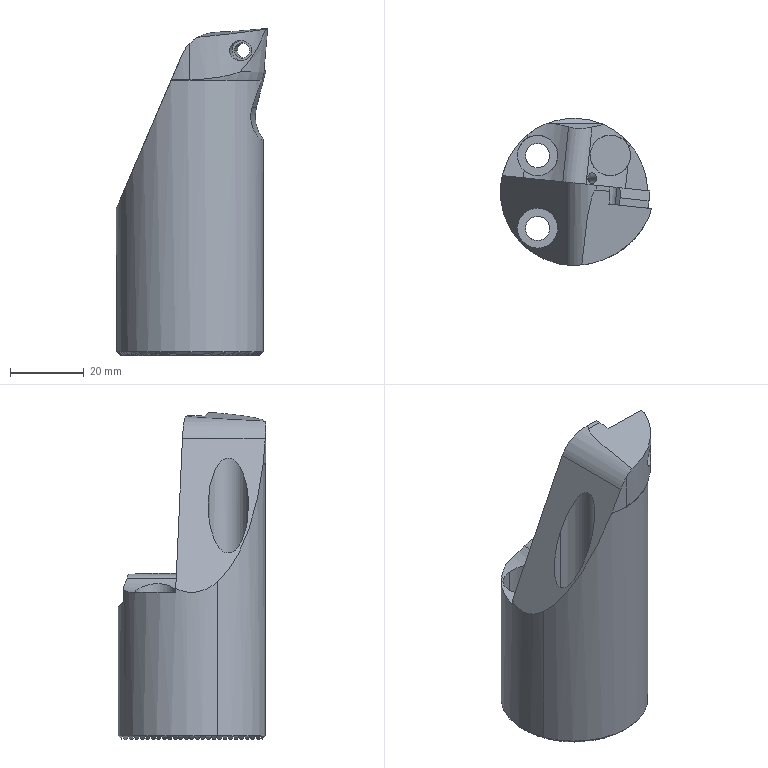NC program | Mastercam | posted with a generic post
Whole program:
%
:0001()
(MATERIAL - ALUMINUM MM - 2024)
(T8|26 60DTH |H8|D8|WEAR COMP|TOOL DIA. - 26.|XY STOCK TO LEAVE - .1|Z STOCK TO LEAVE - -.75)
(T9|12 FEMF |H9|D9|WEAR COMP|TOOL DIA. - 12.|XY STOCK TO LEAVE - .1|Z STOCK TO LEAVE - .05)
(T3|10 CHM |H3)
(T4|12 FEMR |H4|XY STOCK TO LEAVE - .15|Z STOCK TO LEAVE - .1)
N100 G21
N102 G0 G17 G40 G80 G90 G94 G98
N104 G0 G28 G91 Z0.
N106 G0 G28 X0. Y0.
(26 60DTH |TOOL - 8|DIA. OFF. - 8|LEN. - 8|TOOL DIA. - 26.)
N108 T8 M6
N110 G0 G55 G90 X17.402 Y10.083 C0. B-90. S4000 M3
N112 G43 H8 Z70.25
N114 Z21.25
N116 G1 Z14.5 F2000.
N118 G41 D8 X12.473 F1000.
N120 G3 X12.35 Y9.96 J-.123
N122 G1 Y6.96
N124 Y-6.96
N126 Y-9.96
N128 G3 X12.473 Y-10.083 I.123
N130 G1 G40 X17.402
N132 X17.352
N134 G42 D8 X12.423
N136 G2 X12.3 Y-9.96 J.123
N138 G1 Y-6.96
N140 Y6.96
N142 Y9.96
N144 G2 X12.423 Y10.083 I.123
N146 G1 G40 X17.352
N148 G0 Z30.25
N150 X17.402
N152 Z19.75
N154 G1 Z13. F2000.
N156 G41 D8 X12.473 F1000.
N158 G3 X12.35 Y9.96 J-.123
N160 G1 Y6.96
N162 Y-6.96
N164 Y-9.96
N166 G3 X12.473 Y-10.083 I.123
N168 G1 G40 X17.402
N170 X17.352
N172 G42 D8 X12.423
N174 G2 X12.3 Y-9.96 J.123
N176 G1 Y-6.96
N178 Y6.96
N180 Y9.96
N182 G2 X12.423 Y10.083 I.123
N184 G1 G40 X17.352
N186 G0 Z28.75
N188 X17.402 Y13.244
N190 Z18.25
N192 G1 Z11.5 F2000.
N194 G41 D8 X12.473 F1000.
N196 G3 X12.35 Y13.121 J-.123
N198 G1 Y10.121
N200 Y-10.121
N202 Y-13.121
N204 G3 X12.473 Y-13.244 I.123
N206 G1 G40 X17.402
N208 X17.352
N210 G42 D8 X12.423
N212 G2 X12.3 Y-13.121 J.123
N214 G1 Y-10.121
N216 Y10.121
N218 Y13.121
N220 G2 X12.423 Y13.244 I.123
N222 G1 G40 X17.352
N224 G0 Z27.25
N226 X17.402 Y15.45
N228 Z16.75
N230 G1 Z10. F2000.
N232 G41 D8 X12.473 F1000.
N234 G3 X12.35 Y15.326 J-.124
N236 G1 Y12.326
N238 Y-12.326
N240 Y-15.326
N242 G3 X12.473 Y-15.45 I.123
N244 G1 G40 X17.402
N246 X17.352
N248 G42 D8 X12.423
N250 G2 X12.3 Y-15.326 J.124
N252 G1 Y-12.326
N254 Y12.326
N256 Y15.326
N258 G2 X12.423 Y15.45 I.123
N260 G1 G40 X17.352
N262 G0 Z25.75
N264 X17.402 Y17.157
N266 Z15.25
N268 G1 Z8.5 F2000.
N270 G41 D8 X12.473 F1000.
N272 G3 X12.35 Y17.033 J-.124
N274 G1 Y14.033
N276 Y-14.033
N278 Y-17.033
N280 G3 X12.473 Y-17.157 I.123
N282 G1 G40 X17.402
N284 X17.352
N286 G42 D8 X12.423
N288 G2 X12.3 Y-17.033 J.124
N290 G1 Y-14.033
N292 Y14.033
N294 Y17.033
N296 G2 X12.423 Y17.157 I.123
N298 G1 G40 X17.352
N300 G0 Z24.25
N302 X17.402 Y18.532
N304 Z13.75
N306 G1 Z7. F2000.
N308 G41 D8 X12.473 F1000.
N310 G3 X12.35 Y18.409 J-.123
N312 G1 Y15.409
N314 Y-15.409
N316 Y-18.409
N318 G3 X12.473 Y-18.532 I.123
N320 G1 G40 X17.402
N322 X17.352
N324 G42 D8 X12.423
N326 G2 X12.3 Y-18.409 J.123
N328 G1 Y-15.409
N330 Y15.409
N332 Y18.409
N334 G2 X12.423 Y18.532 I.123
N336 G1 G40 X17.352
N338 G0 Z22.75
N340 X17.402 Y19.659
N342 Z12.25
N344 G1 Z5.5 F2000.
N346 G41 D8 X12.473 F1000.
N348 G3 X12.35 Y19.536 J-.123
N350 G1 Y16.536
N352 Y-16.536
N354 Y-19.536
N356 G3 X12.473 Y-19.659 I.123
N358 G1 G40 X17.402
N360 X17.352
N362 G42 D8 X12.423
N364 G2 X12.3 Y-19.536 J.123
N366 G1 Y-16.536
N368 Y16.536
N370 Y19.536
N372 G2 X12.423 Y19.659 I.123
N374 G1 G40 X17.352
N376 G0 Z21.25
N378 X17.402 Y20.586
N380 Z10.75
N382 G1 Z4. F2000.
N384 G41 D8 X12.473 F1000.
N386 G3 X12.35 Y20.462 J-.124
N388 G1 Y17.462
N390 Y-17.462
N392 Y-20.462
N394 G3 X12.473 Y-20.586 I.123
N396 G1 G40 X17.402
N398 X17.352
N400 G42 D8 X12.423
N402 G2 X12.3 Y-20.462 J.124
N404 G1 Y-17.462
N406 Y17.462
N408 Y20.462
N410 G2 X12.423 Y20.586 I.123
N412 G1 G40 X17.352
N414 G0 Z19.75
N416 X17.402 Y21.342
N418 Z9.25
N420 G1 Z2.5 F2000.
N422 G41 D8 X12.473 F1000.
N424 G3 X12.35 Y21.219 J-.123
N426 G1 Y18.219
N428 Y-18.219
N430 Y-21.219
N432 G3 X12.473 Y-21.342 I.123
N434 G1 G40 X17.402
N436 X17.352
N438 G42 D8 X12.423
N440 G2 X12.3 Y-21.219 J.123
N442 G1 Y-18.219
N444 Y18.219
N446 Y21.219
N448 G2 X12.423 Y21.342 I.123
N450 G1 G40 X17.352
N452 G0 Z18.25
N454 X17.402 Y21.95
N456 Z7.75
N458 G1 Z1. F2000.
N460 G41 D8 X12.473 F1000.
N462 G3 X12.35 Y21.827 J-.123
N464 G1 Y18.827
N466 Y-18.827
N468 Y-21.827
N470 G3 X12.473 Y-21.95 I.123
N472 G1 G40 X17.402
N474 X17.352
N476 G42 D8 X12.423
N478 G2 X12.3 Y-21.827 J.123
N480 G1 Y-18.827
N482 Y18.827
N484 Y21.827
N486 G2 X12.423 Y21.95 I.123
N488 G1 G40 X17.352
N490 G0 Z16.75
N492 X17.402 Y22.422
N494 Z6.25
N496 G1 Z-.5 F2000.
N498 G41 D8 X12.473 F1000.
N500 G3 X12.35 Y22.299 J-.123
N502 G1 Y19.299
N504 Y-19.299
N506 Y-22.299
N508 G3 X12.473 Y-22.422 I.123
N510 G1 G40 X17.402
N512 X17.352
N514 G42 D8 X12.423
N516 G2 X12.3 Y-22.299 J.123
N518 G1 Y-19.299
N520 Y19.299
N522 Y22.299
N524 G2 X12.423 Y22.422 I.123
N526 G1 G40 X17.352
N528 G0 Z15.25
N530 X17.402 Y22.769
N532 Z4.75
N534 G1 Z-2. F2000.
N536 G41 D8 X12.473 F1000.
N538 G3 X12.35 Y22.645 J-.124
N540 G1 Y19.645
N542 Y-19.645
N544 Y-22.645
N546 G3 X12.473 Y-22.769 I.123
N548 G1 G40 X17.402
N550 X17.352
N552 G42 D8 X12.423
N554 G2 X12.3 Y-22.645 J.124
N556 G1 Y-19.645
N558 Y19.645
N560 Y22.645
N562 G2 X12.423 Y22.769 I.123
N564 G1 G40 X17.352
N566 G0 Z13.75
N568 X17.402 Y22.996
N570 Z3.25
N572 G1 Z-3.5 F2000.
N574 G41 D8 X12.473 F1000.
N576 G3 X12.35 Y22.873 J-.123
N578 G1 Y19.873
N580 Y-19.873
N582 Y-22.873
N584 G3 X12.473 Y-22.996 I.123
N586 G1 G40 X17.402
N588 X17.352
N590 G42 D8 X12.423
N592 G2 X12.3 Y-22.873 J.123
N594 G1 Y-19.873
N596 Y19.873
N598 Y22.873
N600 G2 X12.423 Y22.996 I.123
N602 G1 G40 X17.352
N604 G0 Z12.25
N606 X17.402 Y23.109
N608 Z1.75
N610 G1 Z-5. F2000.
N612 G41 D8 X12.473 F1000.
N614 G3 X12.35 Y22.986 J-.123
N616 G1 Y19.986
N618 Y-19.986
N620 Y-22.986
N622 G3 X12.473 Y-23.109 I.123
N624 G1 G40 X17.402
N626 X17.352
N628 G42 D8 X12.423
N630 G2 X12.3 Y-22.986 J.123
N632 G1 Y-19.986
N634 Y19.986
N636 Y22.986
N638 G2 X12.423 Y23.109 I.123
N640 G1 G40 X17.352
N642 G0 Z10.75
N644 X17.402
N646 Z.25
N648 G1 Z-6.5 F2000.
N650 G41 D8 X12.473 F1000.
N652 G3 X12.35 Y22.986 J-.123
N654 G1 Y19.986
N656 Y-19.986
N658 Y-22.986
N660 G3 X12.473 Y-23.109 I.123
N662 G1 G40 X17.402
N664 X17.352
N666 G42 D8 X12.423
N668 G2 X12.3 Y-22.986 J.123
N670 G1 Y-19.986
N672 Y19.986
N674 Y22.986
N676 G2 X12.423 Y23.109 I.123
N678 G1 G40 X17.352
N680 G0 Z9.25
N682 X17.402 Y22.996
N684 Z-1.25
N686 G1 Z-8. F2000.
N688 G41 D8 X12.473 F1000.
N690 G3 X12.35 Y22.873 J-.123
N692 G1 Y19.873
N694 Y-19.873
N696 Y-22.873
N698 G3 X12.473 Y-22.996 I.123
N700 G1 G40 X17.402
N702 X17.352
N704 G42 D8 X12.423
N706 G2 X12.3 Y-22.873 J.123
N708 G1 Y-19.873
N710 Y19.873
N712 Y22.873
N714 G2 X12.423 Y22.996 I.123
N716 G1 G40 X17.352
N718 G0 Z7.75
N720 X17.402 Y22.769
N722 Z-2.75
N724 G1 Z-9.5 F2000.
N726 G41 D8 X12.473 F1000.
N728 G3 X12.35 Y22.645 J-.124
N730 G1 Y19.645
N732 Y-19.645
N734 Y-22.645
N736 G3 X12.473 Y-22.769 I.123
N738 G1 G40 X17.402
N740 X17.352
N742 G42 D8 X12.423
N744 G2 X12.3 Y-22.645 J.124
N746 G1 Y-19.645
N748 Y19.645
N750 Y22.645
N752 G2 X12.423 Y22.769 I.123
N754 G1 G40 X17.352
N756 G0 Z6.25
N758 X17.402 Y22.422
N760 Z-4.25
N762 G1 Z-11. F2000.
N764 G41 D8 X12.473 F1000.
N766 G3 X12.35 Y22.299 J-.123
N768 G1 Y19.299
N770 Y-19.299
N772 Y-22.299
N774 G3 X12.473 Y-22.422 I.123
N776 G1 G40 X17.402
N778 X17.352
N780 G42 D8 X12.423
N782 G2 X12.3 Y-22.299 J.123
N784 G1 Y-19.299
N786 Y19.299
N788 Y22.299
N790 G2 X12.423 Y22.422 I.123
N792 G1 G40 X17.352
N794 G0 Z4.75
N796 X17.402 Y21.95
N798 Z-5.75
N800 G1 Z-12.5 F2000.
N802 G41 D8 X12.473 F1000.
N804 G3 X12.35 Y21.827 J-.123
N806 G1 Y18.827
N808 Y-18.827
N810 Y-21.827
N812 G3 X12.473 Y-21.95 I.123
N814 G1 G40 X17.402
N816 X17.352
N818 G42 D8 X12.423
N820 G2 X12.3 Y-21.827 J.123
N822 G1 Y-18.827
N824 Y18.827
N826 Y21.827
N828 G2 X12.423 Y21.95 I.123
N830 G1 G40 X17.352
N832 G0 Z3.25
N834 X17.402 Y21.342
N836 Z-7.25
N838 G1 Z-14. F2000.
N840 G41 D8 X12.473 F1000.
N842 G3 X12.35 Y21.219 J-.123
N844 G1 Y18.219
N846 Y-18.219
N848 Y-21.219
N850 G3 X12.473 Y-21.342 I.123
N852 G1 G40 X17.402
N854 X17.352
N856 G42 D8 X12.423
N858 G2 X12.3 Y-21.219 J.123
N860 G1 Y-18.219
N862 Y18.219
N864 Y21.219
N866 G2 X12.423 Y21.342 I.123
N868 G1 G40 X17.352
N870 G0 Z1.75
N872 X17.402 Y20.586
N874 Z-8.75
N876 G1 Z-15.5 F2000.
N878 G41 D8 X12.473 F1000.
N880 G3 X12.35 Y20.462 J-.124
N882 G1 Y17.462
N884 Y-17.462
N886 Y-20.462
N888 G3 X12.473 Y-20.586 I.123
N890 G1 G40 X17.402
N892 X17.352
N894 G42 D8 X12.423
N896 G2 X12.3 Y-20.462 J.124
N898 G1 Y-17.462
N900 Y17.462
N902 Y20.462
N904 G2 X12.423 Y20.586 I.123
N906 G1 G40 X17.352
N908 G0 Z.25
N910 X17.402 Y19.659
N912 Z-10.25
N914 G1 Z-17. F2000.
N916 G41 D8 X12.473 F1000.
N918 G3 X12.35 Y19.536 J-.123
N920 G1 Y16.536
N922 Y-16.536
N924 Y-19.536
N926 G3 X12.473 Y-19.659 I.123
N928 G1 G40 X17.402
N930 X17.352
N932 G42 D8 X12.423
N934 G2 X12.3 Y-19.536 J.123
N936 G1 Y-16.536
N938 Y16.536
N940 Y19.536
N942 G2 X12.423 Y19.659 I.123
N944 G1 G40 X17.352
N946 G0 Z-1.25
N948 X17.402 Y18.532
N950 Z-11.75
N952 G1 Z-18.5 F2000.
N954 G41 D8 X12.473 F1000.
N956 G3 X12.35 Y18.409 J-.123
N958 G1 Y15.409
N960 Y-15.409
N962 Y-18.409
N964 G3 X12.473 Y-18.532 I.123
N966 G1 G40 X17.402
N968 X17.352
N970 G42 D8 X12.423
N972 G2 X12.3 Y-18.409 J.123
N974 G1 Y-15.409
N976 Y15.409
N978 Y18.409
N980 G2 X12.423 Y18.532 I.123
N982 G1 G40 X17.352
N984 G0 Z-2.75
N986 X17.402 Y17.157
N988 Z-13.25
N990 G1 Z-20. F2000.
N992 G41 D8 X12.473 F1000.
N994 G3 X12.35 Y17.033 J-.124
N996 G1 Y14.033
N998 Y-14.033
N1000 Y-17.033
N1002 G3 X12.473 Y-17.157 I.123
N1004 G1 G40 X17.402
N1006 X17.352
N1008 G42 D8 X12.423
N1010 G2 X12.3 Y-17.033 J.124
N1012 G1 Y-14.033
N1014 Y14.033
N1016 Y17.033
N1018 G2 X12.423 Y17.157 I.123
N1020 G1 G40 X17.352
N1022 G0 Z-4.25
N1024 X17.402 Y15.45
N1026 Z-14.75
N1028 G1 Z-21.5 F2000.
N1030 G41 D8 X12.473 F1000.
N1032 G3 X12.35 Y15.326 J-.124
N1034 G1 Y12.326
N1036 Y-12.326
N1038 Y-15.326
N1040 G3 X12.473 Y-15.45 I.123
N1042 G1 G40 X17.402
N1044 X17.352
N1046 G42 D8 X12.423
N1048 G2 X12.3 Y-15.326 J.124
N1050 G1 Y-12.326
N1052 Y12.326
N1054 Y15.326
N1056 G2 X12.423 Y15.45 I.123
N1058 G1 G40 X17.352
N1060 G0 Z-5.75
N1062 X17.402 Y13.244
N1064 Z-16.25
N1066 G1 Z-23. F2000.
N1068 G41 D8 X12.473 F1000.
N1070 G3 X12.35 Y13.121 J-.123
N1072 G1 Y10.121
N1074 Y-10.121
N1076 Y-13.121
N1078 G3 X12.473 Y-13.244 I.123
N1080 G1 G40 X17.402
N1082 X17.352
N1084 G42 D8 X12.423
N1086 G2 X12.3 Y-13.121 J.123
N1088 G1 Y-10.121
N1090 Y10.121
N1092 Y13.121
N1094 G2 X12.423 Y13.244 I.123
N1096 G1 G40 X17.352
N1098 G0 Z-7.25
N1100 X17.402 Y10.083
N1102 Z-17.75
N1104 G1 Z-24.5 F2000.
N1106 G41 D8 X12.473 F1000.
N1108 G3 X12.35 Y9.96 J-.123
N1110 G1 Y6.96
N1112 Y-6.96
N1114 Y-9.96
N1116 G3 X12.473 Y-10.083 I.123
N1118 G1 G40 X17.402
N1120 X17.352
N1122 G42 D8 X12.423
N1124 G2 X12.3 Y-9.96 J.123
N1126 G1 Y-6.96
N1128 Y6.96
N1130 Y9.96
N1132 G2 X12.423 Y10.083 I.123
N1134 G1 G40 X17.352
N1136 G0 Z31.25
N1138 M5
N1140 G0 G28 G91 Z0.
N1142 G28 B0.
N1144 M01
N1146 G0 G17 G40 G80 G90 G94 G98
N1148 G0 G28 G91 Z0.
(12 FEMF |TOOL - 9|DIA. OFF. - 9|LEN. - 9|TOOL DIA. - 12.)
N1150 T9 M6
N1152 G0 G55 G90 X-33.9 Y22.071 C0. B-90. S3500 M3
N1154 G43 H9 Z84.5
N1156 Z35.5
N1158 G1 Z34.008 F2000.
N1160 G41 D9 Y14.071 F1500.
N1162 Y-14.071
N1164 G40 Y-22.071
N1166 Z33.517 F2000.
N1168 G42 D9 Y-14.071 F1500.
N1170 Y14.071
N1172 G40 Y22.071
N1174 Z33.025 F2000.
N1176 G41 D9 Y14.071 F1500.
N1178 Y-14.071
N1180 G40 Y-22.071
N1182 Z32.533 F2000.
N1184 G42 D9 Y-14.071 F1500.
N1186 Y14.071
N1188 G40 Y22.071
N1190 Z32.042 F2000.
N1192 G41 D9 Y14.071 F1500.
N1194 Y-14.071
N1196 G40 Y-22.071
N1198 Z31.55 F2000.
N1200 G42 D9 Y-14.071 F1500.
N1202 Y14.071
N1204 G40 Y22.071
N1206 G0 Z84.5
N1208 X-34.
N1210 Z35.5
N1212 G1 Z31.5 F2000.
N1214 G41 D9 Y14.071 F600.
N1216 Y-14.071
N1218 G40 Y-22.071
N1220 G0 Z84.5
N1222 M5
N1224 G0 G28 G91 Z0.
N1226 G28 B0.
N1228 M01
N1230 G0 G17 G40 G80 G90 G94 G98
N1232 G0 G28 G91 Z0.
(10 CHM |TOOL - 3|DIA. OFF. - 3|LEN. - 3|TOOL DIA. - 10.)
N1234 M8
N1236 T3 M6
N1238 G0 G55 G90 X0. Y27.4 C0. B0. S3000 M3
N1240 G43 H3 Z50.
N1242 G81 G98 Z-3. R1. F300.
N1244 X-23.729 Y-13.7
N1246 X23.729
N1248 G80
N1250 M9
N1252 M5
N1254 G0 G28 G91 Z0.
N1256 G28
N1258 M01
N1260 G0 G17 G40 G80 G90 G94 G98
N1262 G0 G28 G91 Z0.
(12 FEMR |TOOL - 4|DIA. OFF. - 4|LEN. - 4|TOOL DIA. - 12.)
N1264 M8
N1266 T4 M6
N1268 G0 G55 G90 X4.567 Y-2.882 C0. B0. S5500 M3
N1270 G43 H4 Z50.
N1272 Z3.
N1274 G3 X5.4 Y0. Z2.894 I-4.567 J2.882 F2000.
N1276 X0. Y5.4 Z2.598 I-5.4
N1278 X-5.4 Y0. Z2.301 J-5.4
N1280 X0. Y-5.4 Z2.005 I5.4
N1282 X5.4 Y0. Z1.709 J5.4
N1284 X0. Y5.4 Z1.413 I-5.4
N1286 X-5.4 Y0. Z1.117 J-5.4
N1288 X0. Y-5.4 Z.82 I5.4
N1290 X5.4 Y0. Z.524 J5.4
N1292 X0. Y5.4 Z.228 I-5.4
N1294 X-5.4 Y0. Z-.068 J-5.4
N1296 X0. Y-5.4 Z-.364 I5.4
N1298 X5.4 Y0. Z-.661 J5.4
N1300 X0. Y5.4 Z-.957 I-5.4
N1302 X-5.4 Y0. Z-1.253 J-5.4
N1304 X0. Y-5.4 Z-1.549 I5.4
N1306 X5.4 Y0. Z-1.845 J5.4
N1308 X0. Y5.4 Z-2.142 I-5.4
N1310 X-5.4 Y0. Z-2.438 J-5.4
N1312 X0. Y-5.4 Z-2.734 I5.4
N1314 X5.4 Y0. Z-3.03 J5.4
N1316 X0. Y5.4 Z-3.327 I-5.4
N1318 X-5.4 Y0. Z-3.623 J-5.4
N1320 X0. Y-5.4 Z-3.919 I5.4
N1322 X5.4 Y0. Z-4.215 J5.4
N1324 X0. Y5.4 Z-4.511 I-5.4
N1326 X-5.4 Y0. Z-4.808 J-5.4
N1328 X0. Y-5.4 Z-5.104 I5.4
N1330 X5.4 Y0. Z-5.4 J5.4
N1332 X0. Y5.4 I-5.4
N1334 X-5.4 Y0. J-5.4
N1336 X0. Y-5.4 I5.4
N1338 X5.4 Y0. J5.4
N1340 X4.2 Y1.2 Z-5.275 I-1.2
N1342 X3. Y0. Z-5.15 J-1.2
N1344 X4.2 Y-1.2 Z-5.275 I1.2 F4000.
N1346 X5.4 Y0. Z-5.4 J1.2
N1348 X5.408 Y.268 I-4.689 J.268
N1350 X4.953 Y2.284 I-4.697
N1352 X-.045 Y5.493 I-4.998 J-2.287
N1354 X-5.456 Y.961 J-5.496
N1356 X-5.542 Y-.018 I5.499 J-.979
N1358 X.043 Y-5.603 I5.585
N1360 X4.042 Y-3.916 J5.585
N1362 X5.662 Y.075 I-4.106 J3.991
N1364 X5.219 Y2.283 I-5.726
N1366 X-.046 Y5.738 I-5.265 J-2.284
N1368 X-5.533 Y1.684 J-5.739
N1370 X-5.789 Y-.024 I5.574 J-1.708
N1372 X.041 Y-5.854 I5.83
N1374 G1 X.59 Y-5.828
N1376 X1.135 Y-5.75
N1378 X1.67 Y-5.622
N1380 X2.19 Y-5.443
N1382 X2.691 Y-5.217
N1384 X3.168 Y-4.944
N1386 X3.618 Y-4.627
N1388 G3 X5.919 Y.065 I-3.628 J4.691
N1390 X-.011 Y5.995 I-5.93
N1392 X-.859 Y5.935 J-5.93
N1394 X-6.047 Y-.047 I.855 J-5.982
N1396 X-2.781 Y-5.414 I6.043
N1398 X.035 Y-6.099 I2.816 J5.45
N1400 X6.099 Y-.887 J6.135
N1402 X6.171 Y.056 I-6.124 J.943
N1404 X-.025 Y6.252 I-6.196
N1406 X-1.25 Y6.13 J-6.196
N1408 X-6.305 Y-.048 I1.248 J-6.178
N1410 X-2.677 Y-5.755 I6.303
N1412 X.034 Y-6.358 I2.711 J5.795
N1414 X6.389 Y-.705 J6.398
N1416 X6.433 Y.05 I-6.422 J.755
N1418 X-.033 Y6.516 I-6.466
N1420 X-2.185 Y6.148 J-6.466
N1422 X-6.57 Y-.049 I2.187 J-6.197
N1424 X-1.825 Y-6.362 I6.572
N1426 X.026 Y-6.624 I1.851 J6.417
N1428 X6.705 Y.055 J6.679
N1430 X6.689 Y.507 I-6.679
N1432 X-.043 Y6.784 I-6.732 J-.471
N1434 X-3.785 Y5.652 J-6.748
N1436 X-6.838 Y-.049 I3.796 J-5.701
N1438 X-.358 Y-6.888 I6.849
N1440 X.013 Y-6.898 I.371 J6.957
N1442 X6.98 Y.069 J6.967
N1444 X3.385 Y6.165 I-6.967
N1446 X-.041 Y7.049 I-3.426 J-6.194
N1448 X-7.119 Y-.029 J-7.078
N1450 X-6.704 Y-2.418 I7.078
N1452 X.051 Y-7.176 I6.755 J2.416
N1454 X6.348 Y-3.439 J7.174
N1456 X7.245 Y.06 I-6.377 J3.499
N1458 X-.029 Y7.334 I-7.274
N1460 X-1.268 Y7.227 J-7.274
N1462 X-7.392 Y-.051 I1.263 J-7.278
N1464 X-3.58 Y-6.515 I7.387
N1466 X.039 Y-7.447 I3.619 J6.56
N1468 X7.511 Y-.504 J7.492
N1470 X7.531 Y.044 I-7.554 J.548
N1472 X-.043 Y7.618 I-7.574
N1474 X-3.557 Y6.753 J-7.574
N1476 X-7.676 Y-.052 I3.561 J-6.805
N1478 X-1.644 Y-7.553 I7.68
N1480 X.022 Y-7.733 I1.666 J7.618
N1482 X7.82 Y.065 J7.798
N1484 X6.861 Y3.813 I-7.798
N1486 X-.055 Y7.9 I-6.916 J-3.809
N1488 X-7.328 Y3.077 J-7.896
N1490 X-7.958 Y-.034 I7.369 J-3.111
N1492 X.041 Y-8.033 I7.999
N1494 X3.502 Y-7.244 J7.999
N1496 X8.106 Y.073 I-3.513 J7.317
N1498 X.299 Y8.184 I-8.117
N1500 X-.019 Y8.19 I-.318 J-8.233
N1502 X-8.258 Y-.049 J-8.239
N1504 X-5.773 Y-5.948 I8.239
N1506 X.052 Y-8.319 I5.825 J5.971
N1508 X8.154 Y-1.966 J8.342
N1510 X8.399 Y.053 I-8.194 J2.019
N1512 X-.04 Y8.492 I-8.439
N1514 X-3.102 Y7.917 J-8.439
N1516 X-8.553 Y-.054 I3.102 J-7.971
N1518 X-2.969 Y-8.075 I8.553
N1520 X.038 Y-8.613 I3.007 J8.129
N1522 X8.705 Y.054 J8.667
N1524 G1 X8.688 Y.603
N1526 X8.636 Y1.151
N1528 X8.549 Y1.693
N1530 X8.428 Y2.23
N1532 G3 X-.056 Y8.789 I-8.485 J-2.209
N1534 X-6.801 Y5.624 J-8.768
N1536 X-8.851 Y-.049 I6.825 J-5.673
N1538 X.024 Y-8.924 I8.875
N1540 X1.165 Y-8.85 J8.875
N1542 X9.005 Y.076 I-1.161 J8.926
N1544 X3.737 Y8.266 I-9.001
N1546 X-.041 Y9.085 I-3.778 J-8.303
N1548 X-9.163 Y-.037 J-9.122
N1550 X-8.69 Y-2.936 I9.122
N1552 X.057 Y-9.227 I8.747 J2.936
N1554 X7.661 Y-5.227 J9.227
N1556 X9.309 Y.069 I-7.686 J5.296
N1558 X-.025 Y9.403 I-9.334
N1560 X-1.377 Y9.305 J-9.334
N1562 X-9.469 Y-.055 I1.367 J-9.36
N1564 X-5.431 Y-7.807 I9.459
N1566 X.051 Y-9.533 I5.482 J7.845
N1568 X9.596 Y-.666 J9.571
N1570 X9.622 Y.044 I-9.646 J.71
N1572 X-.05 Y9.716 I-9.672
N1574 X-4.975 Y8.368 J-9.672
N1576 X-9.781 Y-.056 I4.98 J-8.424
N1578 X-2.343 Y-9.557 I9.786
N1580 X.003 Y-9.841 I2.346 J9.561
N1582 X9.848 Y.004 J9.845
N1584 X2.443 Y9.542 I-9.845
N1586 X0. Y9.85 I-2.443 J-9.542
N1588 X-9.85 Y0. J-9.85
N1590 X-2.608 Y-9.498 I9.85
N1592 X-.113 Y-9.849 I2.608 J9.498
N1594 G1 X-.082 Z-5.397
N1596 G3 X1.805 Y-9.08 Z-5.208 J2.699
N1598 G1 X2.269 Y-8.628 Z-5.15
N1600 G0 Z50.
N1602 M9
N1604 M5
N1606 G0 G28 G91 Z0.
N1608 G28
N1610 M01
N1612 G0 G17 G40 G80 G90 G94 G98
N1614 G0 G28 G91 Z0.
(12 FEMF |TOOL - 9|DIA. OFF. - 9|LEN. - 9|TOOL DIA. - 12.)
N1616 M8
N1618 T9 M6
N1620 G0 G55 G90 X4.874 Y2.596 C0. B0. S5500 M3
N1622 G43 H9 Z50.
N1624 Z1.
N1626 G1 Z-5.5 F2000.
N1628 G41 D9 X8.22 Y4.788 F600.
N1630 G3 X8.447 Y5.207 I-.274 J.419
N1632 X8.364 Y5.481 I-.501
N1634 X0. Y10. I-8.364 J-5.481
N1636 X-10. Y0. J-10.
N1638 X0. Y-10. I10.
N1640 X10. Y0. J10.
N1642 X8.364 Y5.481 I-10.
N1644 X8.08 Y5.892 I-8.364 J-5.481
N1646 X7.676 Y6.097 I-.404 J-.295
N1648 X7.381 Y6.001 J-.5
N1650 G1 G40 X4.149 Y3.644
N1652 X4.874 Y2.596
N1654 G41 D9 X8.22 Y4.788
N1656 G3 X8.447 Y5.207 I-.274 J.419
N1658 X8.364 Y5.481 I-.501
N1660 X0. Y10. I-8.364 J-5.481
N1662 X-10. Y0. J-10.
N1664 X0. Y-10. I10.
N1666 X10. Y0. J10.
N1668 X8.364 Y5.481 I-10.
N1670 X8.08 Y5.892 I-8.364 J-5.481
N1672 X7.676 Y6.097 I-.404 J-.295
N1674 X7.381 Y6.001 J-.5
N1676 G1 G40 X4.149 Y3.644
N1678 G0 Z50.
N1680 M9
N1682 M5
N1684 G0 G28 G91 Z0.
N1686 G0 G28 X0. Y0.
N1688 G28
N1690 M30
%